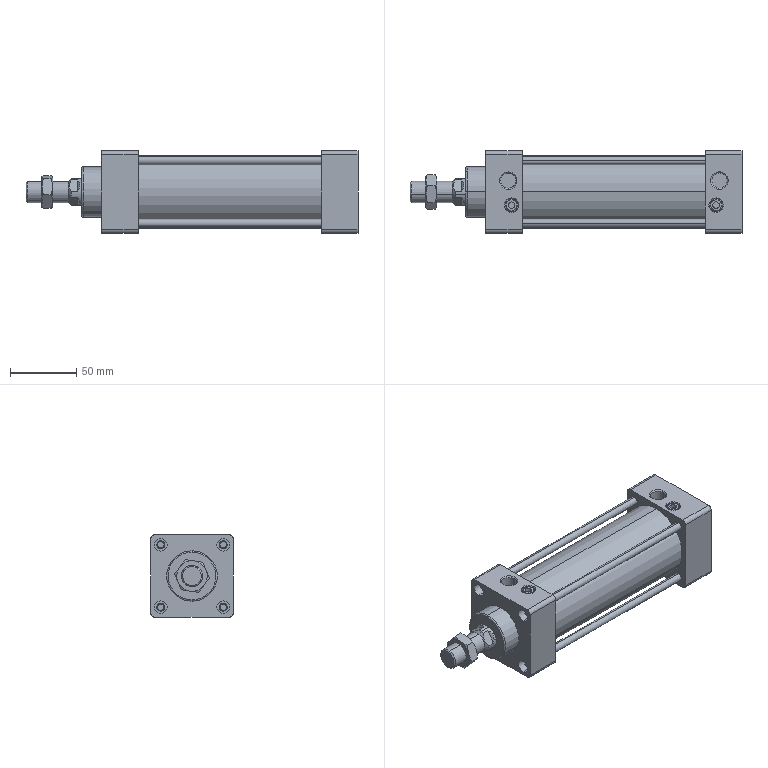Part | SolidWorks | 3 solids | 194 faces | box 250 x 62 x 62 mm | volume 379695 mm3 | cylinder 84 | plane 60 | cone 48 | spline 2 | commonest cylinder face diameters 4.917 x16 6 x16 9.5 x16 5 x4 9.1 x4 10.1 x4